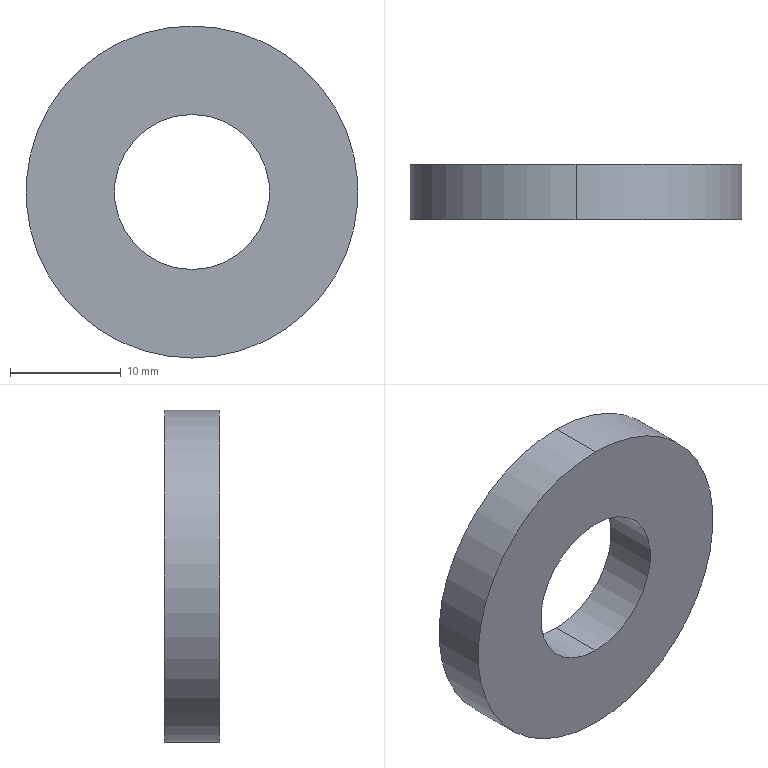Part | Creo | 1 solid | 6 faces | box 30 x 5 x 30 mm | volume 2765 mm3 | cylinder 4 | plane 2 | commonest cylinder face diameters 14 x2 30 x2
STEP:
#1=CARTESIAN_POINT('',(0.,0.,0.));
#2=DIRECTION('',(0.,0.,1.));
#3=DIRECTION('',(1.,0.,0.));
#4=AXIS2_PLACEMENT_3D('',#1,#2,#3);
#5=CARTESIAN_POINT('',(-0.05,375.5,-18.134));
#6=VERTEX_POINT('',#5);
#7=CARTESIAN_POINT('',(-0.05,375.5,-4.133));
#8=VERTEX_POINT('',#7);
#9=CARTESIAN_POINT('',(-0.05,375.5,-11.133));
#10=DIRECTION('',(0.,-1.,0.));
#11=DIRECTION('',(0.,0.,-1.));
#12=AXIS2_PLACEMENT_3D('',#9,#10,#11);
#13=CIRCLE('',#12,7.);
#14=EDGE_CURVE('',#6,#8,#13,.T.);
#15=ORIENTED_EDGE('',*,*,#14,.T.);
#16=CARTESIAN_POINT('',(-0.05,370.5,-4.133));
#17=VERTEX_POINT('',#16);
#18=CARTESIAN_POINT('',(-0.05,375.5,-4.133));
#19=DIRECTION('',(0.,-1.,0.));
#20=VECTOR('',#19,5.);
#21=LINE('',#18,#20);
#22=EDGE_CURVE('',#8,#17,#21,.T.);
#23=ORIENTED_EDGE('',*,*,#22,.T.);
#24=CARTESIAN_POINT('',(-0.05,370.5,-18.134));
#25=VERTEX_POINT('',#24);
#26=CARTESIAN_POINT('',(-0.05,370.5,-11.133));
#27=DIRECTION('',(0.,1.,0.));
#28=DIRECTION('',(0.,0.,1.));
#29=AXIS2_PLACEMENT_3D('',#26,#27,#28);
#30=CIRCLE('',#29,7.);
#31=EDGE_CURVE('',#17,#25,#30,.T.);
#32=ORIENTED_EDGE('',*,*,#31,.T.);
#33=CARTESIAN_POINT('',(-0.05,375.5,-18.134));
#34=DIRECTION('',(0.,-1.,0.));
#35=VECTOR('',#34,5.);
#36=LINE('',#33,#35);
#37=EDGE_CURVE('',#6,#25,#36,.T.);
#38=ORIENTED_EDGE('',*,*,#37,.F.);
#39=EDGE_LOOP('',(#15,#23,#32,#38));
#40=FACE_OUTER_BOUND('',#39,.F.);
#41=CARTESIAN_POINT('',(-0.05,375.5,-11.133));
#42=DIRECTION('',(0.,-1.,0.));
#43=DIRECTION('',(0.,0.,-1.));
#44=AXIS2_PLACEMENT_3D('',#41,#42,#43);
#45=CYLINDRICAL_SURFACE('',#44,7.);
#46=ADVANCED_FACE('',(#40),#45,.F.);
#47=CARTESIAN_POINT('',(-0.05,375.5,3.866));
#48=VERTEX_POINT('',#47);
#49=CARTESIAN_POINT('',(-0.05,375.5,-26.134));
#50=VERTEX_POINT('',#49);
#51=CARTESIAN_POINT('',(-0.05,375.5,-11.133));
#52=DIRECTION('',(0.,1.,0.));
#53=DIRECTION('',(0.,0.,1.));
#54=AXIS2_PLACEMENT_3D('',#51,#52,#53);
#55=CIRCLE('',#54,15.);
#56=EDGE_CURVE('',#48,#50,#55,.T.);
#57=ORIENTED_EDGE('',*,*,#56,.F.);
#58=CARTESIAN_POINT('',(-0.05,375.5,-11.133));
#59=DIRECTION('',(0.,1.,0.));
#60=DIRECTION('',(0.,0.,-1.));
#61=AXIS2_PLACEMENT_3D('',#58,#59,#60);
#62=CIRCLE('',#61,15.);
#63=EDGE_CURVE('',#50,#48,#62,.T.);
#64=ORIENTED_EDGE('',*,*,#63,.F.);
#65=EDGE_LOOP('',(#57,#64));
#66=FACE_OUTER_BOUND('',#65,.F.);
#67=CARTESIAN_POINT('',(-0.05,375.5,-11.133));
#68=DIRECTION('',(0.,-1.,0.));
#69=DIRECTION('',(0.,0.,1.));
#70=AXIS2_PLACEMENT_3D('',#67,#68,#69);
#71=CIRCLE('',#70,7.);
#72=EDGE_CURVE('',#8,#6,#71,.T.);
#73=ORIENTED_EDGE('',*,*,#72,.F.);
#74=ORIENTED_EDGE('',*,*,#14,.F.);
#75=EDGE_LOOP('',(#73,#74));
#76=FACE_BOUND('',#75,.F.);
#77=CARTESIAN_POINT('',(-0.05,375.5,-11.133));
#78=DIRECTION('',(0.,1.,0.));
#79=DIRECTION('',(0.,0.,1.));
#80=AXIS2_PLACEMENT_3D('',#77,#78,#79);
#81=PLANE('',#80);
#82=ADVANCED_FACE('',(#66,#76),#81,.T.);
#83=ORIENTED_EDGE('',*,*,#72,.T.);
#84=ORIENTED_EDGE('',*,*,#37,.T.);
#85=CARTESIAN_POINT('',(-0.05,370.5,-11.133));
#86=DIRECTION('',(0.,1.,0.));
#87=DIRECTION('',(0.,0.,-1.));
#88=AXIS2_PLACEMENT_3D('',#85,#86,#87);
#89=CIRCLE('',#88,7.);
#90=EDGE_CURVE('',#25,#17,#89,.T.);
#91=ORIENTED_EDGE('',*,*,#90,.T.);
#92=ORIENTED_EDGE('',*,*,#22,.F.);
#93=EDGE_LOOP('',(#83,#84,#91,#92));
#94=FACE_OUTER_BOUND('',#93,.F.);
#95=CARTESIAN_POINT('',(-0.05,375.5,-11.133));
#96=DIRECTION('',(0.,-1.,0.));
#97=DIRECTION('',(0.,0.,-1.));
#98=AXIS2_PLACEMENT_3D('',#95,#96,#97);
#99=CYLINDRICAL_SURFACE('',#98,7.);
#100=ADVANCED_FACE('',(#94),#99,.F.);
#101=CARTESIAN_POINT('',(-0.05,370.5,3.866));
#102=VERTEX_POINT('',#101);
#103=CARTESIAN_POINT('',(-0.05,370.5,-26.134));
#104=VERTEX_POINT('',#103);
#105=CARTESIAN_POINT('',(-0.05,370.5,-11.133));
#106=DIRECTION('',(0.,-1.,0.));
#107=DIRECTION('',(0.,0.,1.));
#108=AXIS2_PLACEMENT_3D('',#105,#106,#107);
#109=CIRCLE('',#108,15.);
#110=EDGE_CURVE('',#102,#104,#109,.T.);
#111=ORIENTED_EDGE('',*,*,#110,.F.);
#112=CARTESIAN_POINT('',(-0.05,370.5,-11.133));
#113=DIRECTION('',(0.,-1.,0.));
#114=DIRECTION('',(0.,0.,-1.));
#115=AXIS2_PLACEMENT_3D('',#112,#113,#114);
#116=CIRCLE('',#115,15.);
#117=EDGE_CURVE('',#104,#102,#116,.T.);
#118=ORIENTED_EDGE('',*,*,#117,.F.);
#119=EDGE_LOOP('',(#111,#118));
#120=FACE_OUTER_BOUND('',#119,.F.);
#121=ORIENTED_EDGE('',*,*,#31,.F.);
#122=ORIENTED_EDGE('',*,*,#90,.F.);
#123=EDGE_LOOP('',(#121,#122));
#124=FACE_BOUND('',#123,.F.);
#125=CARTESIAN_POINT('',(-0.05,370.5,-11.133));
#126=DIRECTION('',(0.,1.,0.));
#127=DIRECTION('',(0.,0.,1.));
#128=AXIS2_PLACEMENT_3D('',#125,#126,#127);
#129=PLANE('',#128);
#130=ADVANCED_FACE('',(#120,#124),#129,.F.);
#131=ORIENTED_EDGE('',*,*,#63,.T.);
#132=CARTESIAN_POINT('',(-0.05,375.5,3.866));
#133=DIRECTION('',(0.,-1.,0.));
#134=VECTOR('',#133,5.);
#135=LINE('',#132,#134);
#136=EDGE_CURVE('',#48,#102,#135,.T.);
#137=ORIENTED_EDGE('',*,*,#136,.T.);
#138=ORIENTED_EDGE('',*,*,#110,.T.);
#139=CARTESIAN_POINT('',(-0.05,375.5,-26.134));
#140=DIRECTION('',(0.,-1.,0.));
#141=VECTOR('',#140,5.);
#142=LINE('',#139,#141);
#143=EDGE_CURVE('',#50,#104,#142,.T.);
#144=ORIENTED_EDGE('',*,*,#143,.F.);
#145=EDGE_LOOP('',(#131,#137,#138,#144));
#146=FACE_OUTER_BOUND('',#145,.F.);
#147=CARTESIAN_POINT('',(-0.05,375.5,-11.133));
#148=DIRECTION('',(0.,-1.,0.));
#149=DIRECTION('',(0.,0.,-1.));
#150=AXIS2_PLACEMENT_3D('',#147,#148,#149);
#151=CYLINDRICAL_SURFACE('',#150,15.);
#152=ADVANCED_FACE('',(#146),#151,.T.);
#153=ORIENTED_EDGE('',*,*,#56,.T.);
#154=ORIENTED_EDGE('',*,*,#143,.T.);
#155=ORIENTED_EDGE('',*,*,#117,.T.);
#156=ORIENTED_EDGE('',*,*,#136,.F.);
#157=EDGE_LOOP('',(#153,#154,#155,#156));
#158=FACE_OUTER_BOUND('',#157,.F.);
#159=CARTESIAN_POINT('',(-0.05,375.5,-11.133));
#160=DIRECTION('',(0.,-1.,0.));
#161=DIRECTION('',(0.,0.,-1.));
#162=AXIS2_PLACEMENT_3D('',#159,#160,#161);
#163=CYLINDRICAL_SURFACE('',#162,15.);
#164=ADVANCED_FACE('',(#158),#163,.T.);
#165=CLOSED_SHELL('',(#46,#82,#100,#130,#152,#164));
#166=MANIFOLD_SOLID_BREP('',#165);
#167=(LENGTH_UNIT()NAMED_UNIT(*)SI_UNIT(.MILLI.,.METRE.));
#168=UNCERTAINTY_MEASURE_WITH_UNIT(LENGTH_MEASURE(0.004273),#167,'','');
#169=(NAMED_UNIT(*)PLANE_ANGLE_UNIT()SI_UNIT($,.RADIAN.));
#170=PLANE_ANGLE_MEASURE_WITH_UNIT(PLANE_ANGLE_MEASURE(0.01745),#169);
#171=(CONVERSION_BASED_UNIT('DEGREE',#170)NAMED_UNIT(*)PLANE_ANGLE_UNIT());
#172=(NAMED_UNIT(*)SI_UNIT($,.STERADIAN.)SOLID_ANGLE_UNIT());
#173=(GEOMETRIC_REPRESENTATION_CONTEXT(3)GLOBAL_UNCERTAINTY_ASSIGNED_CONTEXT((#168))GLOBAL_UNIT_ASSIGNED_CONTEXT((#167,#171,#172))REPRESENTATION_CONTEXT('',''));
#174=ADVANCED_BREP_SHAPE_REPRESENTATION('',(#4,#166),#173);